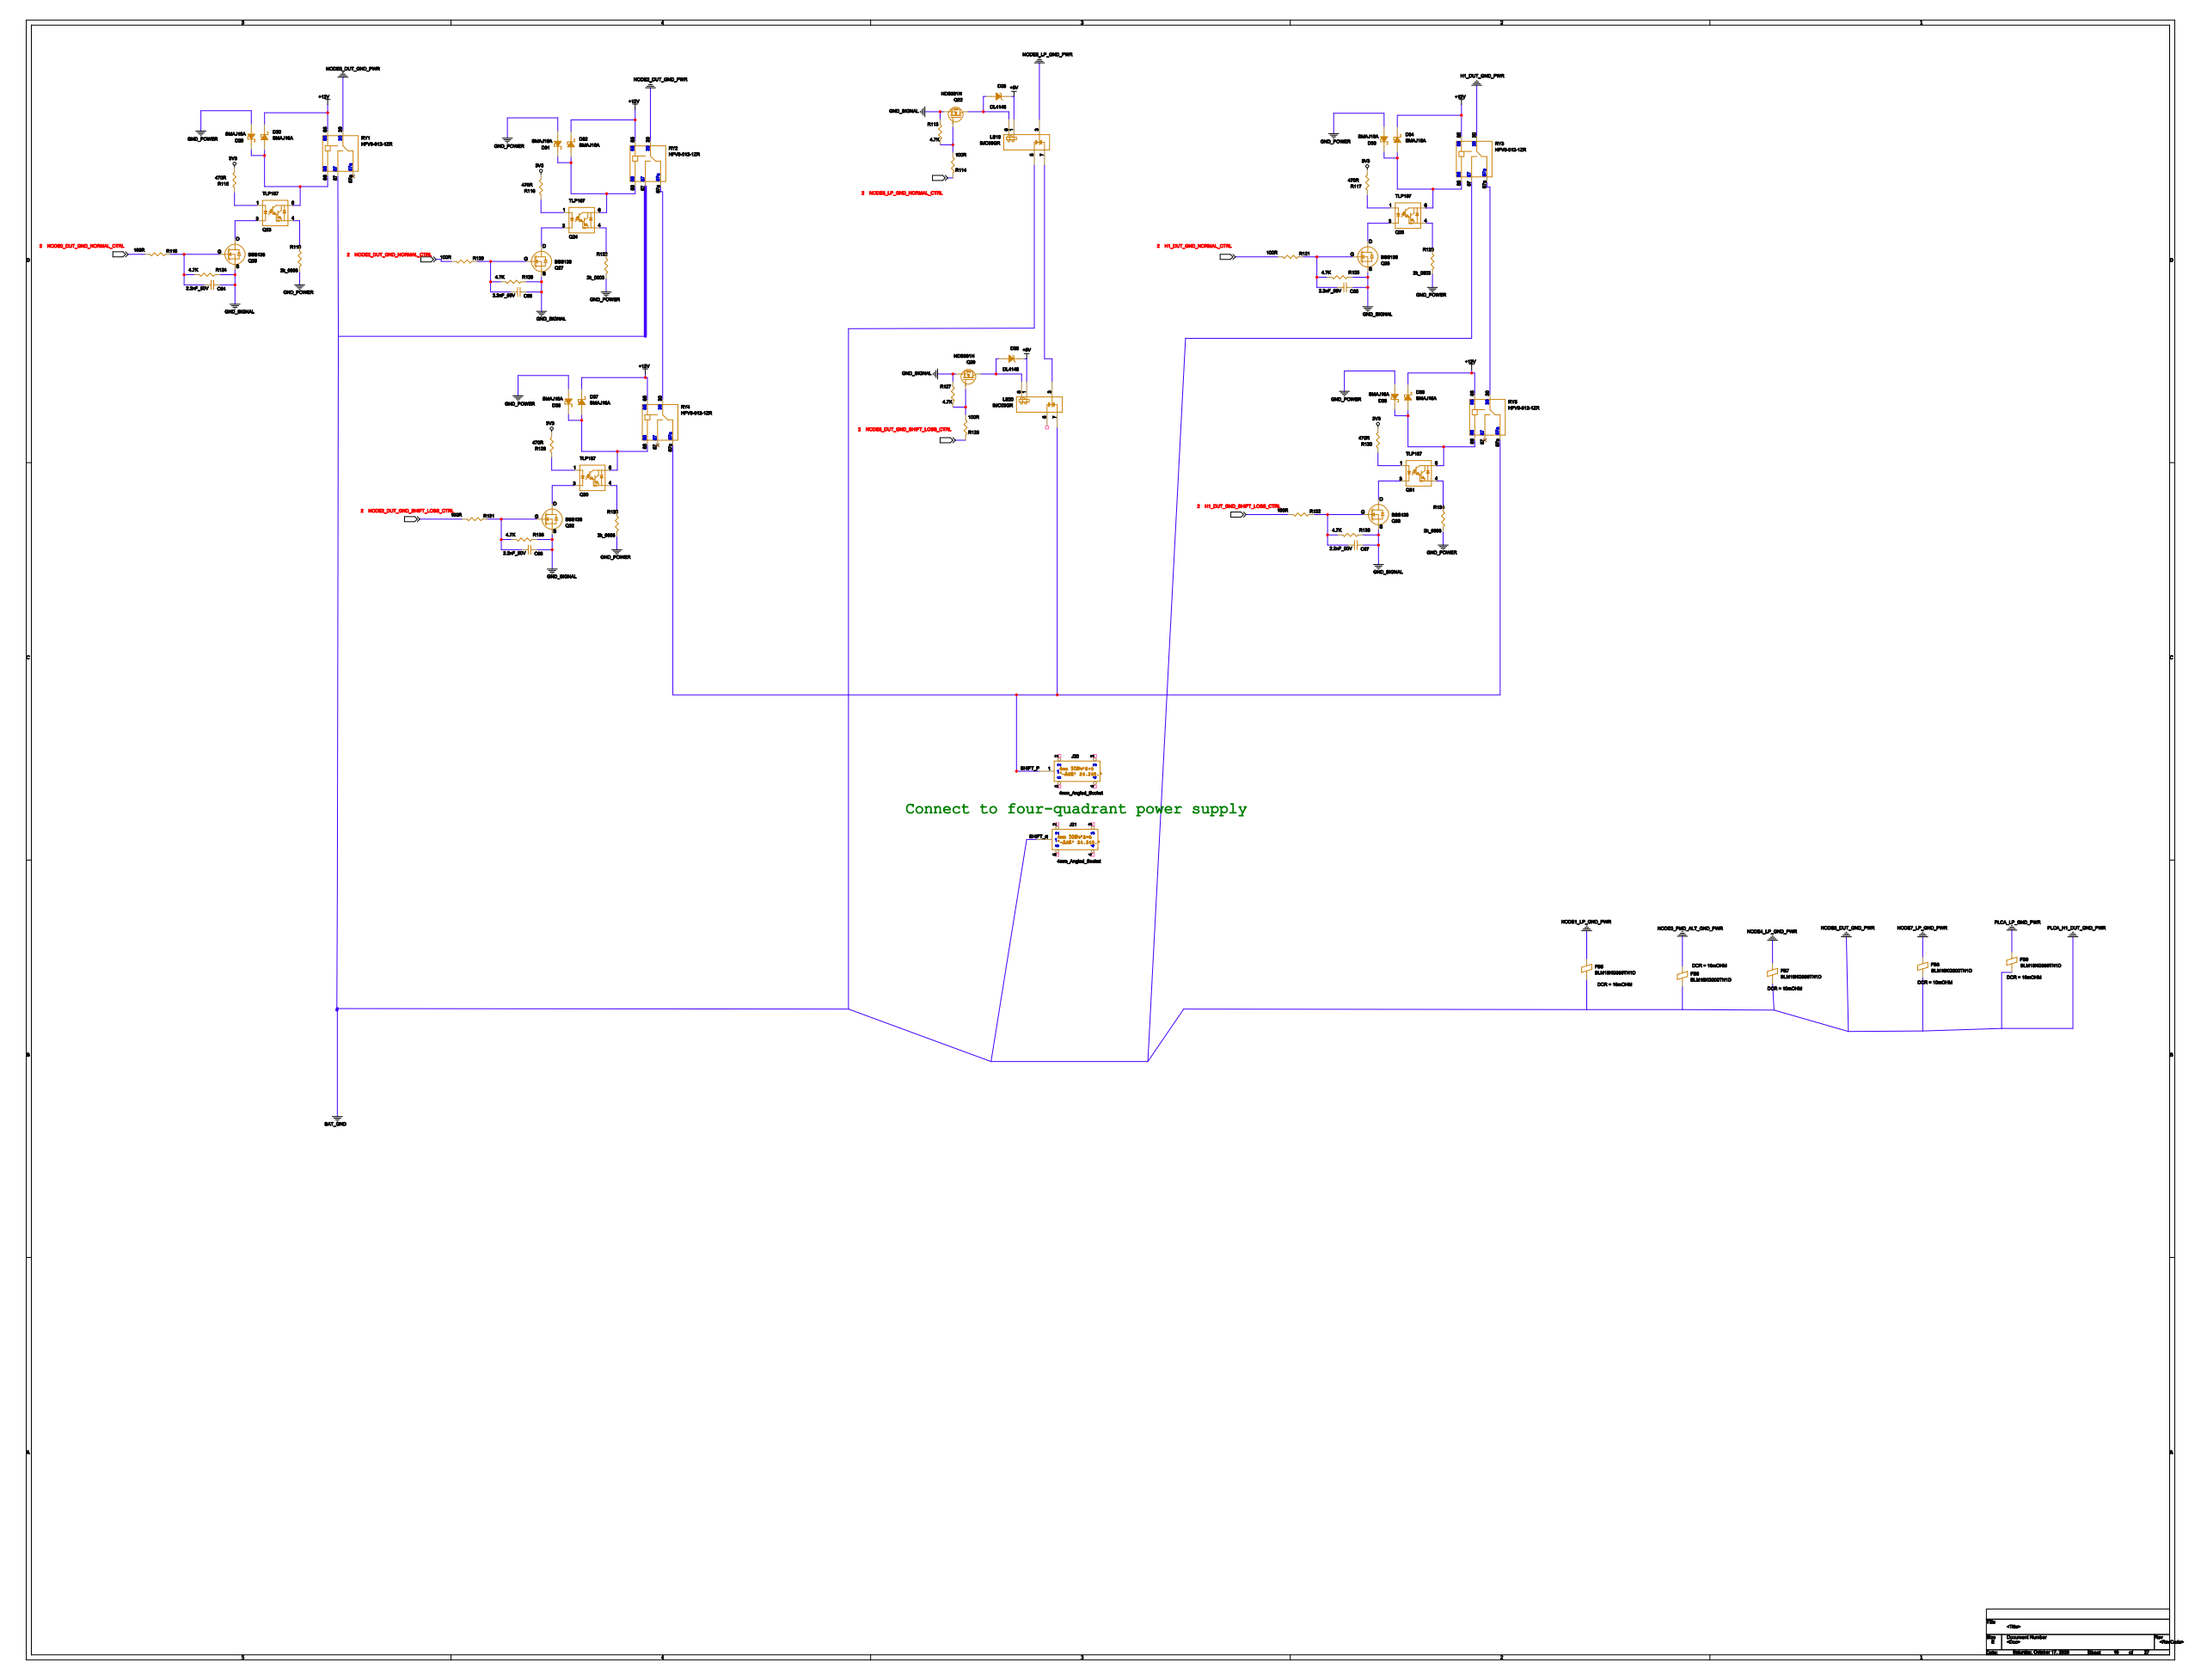Circuit board | Cadence Allegro | 477 parts | 327 nets | one sheet of the schematic
Parts on this sheet (reference | value | footprint):
C64 | 2.2nF_50V | 0603
C65 | 2.2nF_50V | 0603
C66 | 2.2nF_50V | 0603
C67 | 2.2nF_50V | 0603
C68 | 2.2nF_50V | 0603
D28 | DL4148 | MINIMELF
D29 | SMAJ16A | DO-214AC
D30 | SMAJ16A | DO-214AC
D31 | SMAJ16A | DO-214AC
D32 | SMAJ16A | DO-214AC
D33 | SMAJ16A | DO-214AC
D34 | SMAJ16A | DO-214AC
D35 | DL4148 | MINIMELF
D36 | SMAJ16A | DO-214AC
D37 | SMAJ16A | DO-214AC
D38 | SMAJ16A | DO-214AC
D39 | SMAJ16A | DO-214AC
FB5 | BLM18KG300TN1D | 0603
FB6 | BLM18KG300TN1D | 0603
FB7 | BLM18KG300TN1D | 0603
FB8 | BLM18KG300TN1D | 0603
FB9 | BLM18KG300TN1D | 0603
J20 | 4mm_Angled_Socket | YJX40016A
J21 | 4mm_Angled_Socket | YJX40016A
LS19 | IMC03GR | IMC03GR
LS20 | IMC03GR | IMC03GR
Q22 | NDS331N | SOT23-3
Q23 | TLP187 | TLP187
Q24 | TLP187 | TLP187
Q25 | TLP187 | TLP187
Q26 | BSS138 | 003_SOT23B
Q27 | BSS138 | 003_SOT23B
Q28 | BSS138 | 003_SOT23B
Q29 | NDS331N | SOT23-3
Q30 | TLP187 | TLP187
Q31 | TLP187 | TLP187
Q32 | BSS138 | 003_SOT23B
Q33 | BSS138 | 003_SOT23B
R113 | 4.7K | R0402
R114 | 100R | R0402
R115 | 470R | 0402
R116 | 470R | 0402
R117 | 470R | 0402
R118 | 100R | 0402
R119 | 2k_0603 | 0603
R120 | 100R | 0402
R121 | 100R | 0402
R122 | 2k_0603 | 0603
R123 | 2k_0603 | 0603
R124 | 4.7K | 0402
R125 | 4.7K | 0402
R126 | 4.7K | 0402
R127 | 4.7K | R0402
R128 | 100R | R0402
R129 | 470R | 0402
R130 | 470R | 0402
R131 | 100R | 0402
R132 | 100R | 0402
R133 | 2k_0603 | 0603
R134 | 2k_0603 | 0603
R135 | 4.7K | 0402
R136 | 4.7K | 0402
RY1 | HFV9-012-1ZR | HFV9-012-1ZR
RY2 | HFV9-012-1ZR | HFV9-012-1ZR
RY3 | HFV9-012-1ZR | HFV9-012-1ZR
RY4 | HFV9-012-1ZR | HFV9-012-1ZR
RY5 | HFV9-012-1ZR | HFV9-012-1ZR
Nets of these parts (net: part-pin ...):
N16905300: Q22-1 R113-2 R114-1
NODE5_LP_GND_NORMAL_CTRL: R114-2
N16906404: Q29-1 R127-2 R128-1
NODE5_DUT_GND_SHIFT_LOSS_CTRL: R128-2
N16854640: C64-2 Q26-G R118-2 R124-1
BAT_GND: C64-1 C65-1 C66-1 C67-1 C68-1 D29-1 D31-1 D33-1 D36-1 D38-1 J21-1 LS19-5 Q22-2 Q26-S Q27-S Q28-S Q29-2 Q32-S Q33-S R113-1 R119-2 R122-2 R123-2 R124-2 R125-2 R126-2 R127-1 R133-2 R134-2 R135-2 R136-2 RY1-87 RY2-87 RY3-87
N16863116: C65-2 Q28-G R121-2 R125-1
N16859227: C66-2 Q27-G R120-2 R126-1
N16863316: C67-2 Q33-G R132-2 R135-1
N16860030: C68-2 Q32-G R131-2 R136-1
N16854533: Q23-1 R115-1
3V3: R115-2 R116-2 R117-2 R129-2 R130-2
N16859160: Q24-1 R116-1
N16863049: Q25-1 R117-1
N16859963: Q30-1 R129-1
N16863257: Q31-1 R130-1
N16854975: Q23-4 R119-1
N16859192: Q24-4 R122-1
N16863081: Q25-4 R123-1
N16859995: Q30-4 R133-1
N16863289: Q31-4 R134-1
+12V: D30-2 D32-2 D34-2 D37-2 D39-2 RY1-85 RY2-85 RY3-85 RY4-85 RY5-85
N16854978: D29-2 D30-1 Q23-6 RY1-86
N16859132: D31-2 D32-1 Q24-6 RY2-86
N16863017: D33-2 D34-1 Q25-6 RY3-86
N16859935: D36-2 D37-1 Q30-6 RY4-86
N16863229: D38-2 D39-1 Q31-6 RY5-86
NODE0_DUT_GND_PWR: RY1-30
NODE6_DUT_GND_PWR: FB5-2 FB6-2 FB7-2 FB8-2 FB9-2
SHIFT_P: J20-1 LS20-7 RY4-87A RY5-87A
H1_DUT_GND_PWR: RY3-30
NODE2_DUT_GND_PWR: RY2-30
N16854691: Q23-3 Q26-D
N16859188: Q24-3 Q27-D
N16863077: Q25-3 Q28-D
N16859991: Q30-3 Q32-D
N16863285: Q31-3 Q33-D
N16860773: RY2-87A RY4-30
N16863041: RY3-87A RY5-30
+5V: D28-2 D35-2 LS19-1 LS20-1
N16905267: D28-1 LS19-8 Q22-3
N16906362: D35-1 LS20-8 Q29-3
NODE5_LP_GND_PWR: LS19-3
NODE7_LP_GND_PWR: FB8-1
PLCA_LP_GND_PWR: FB9-1
NODE1_LP_GND_PWR: FB5-1
NODE3_PMD_ALT_GND_PWR: FB6-1
NODE4_LP_GND_PWR: FB7-1
N16906129: LS19-7 LS20-3
NODE0_DUT_GND_NORMAL_CTRL: R118-1
NODE2_DUT_GND_SHIFT_LOSS_CTRL: R131-1
NODE2_DUT_GND_NORMAL_CTRL: R120-1
H1_DUT_GND_NORMAL_CTRL: R121-1
H1_DUT_GND_SHIFT_LOSS_CTRL: R132-1